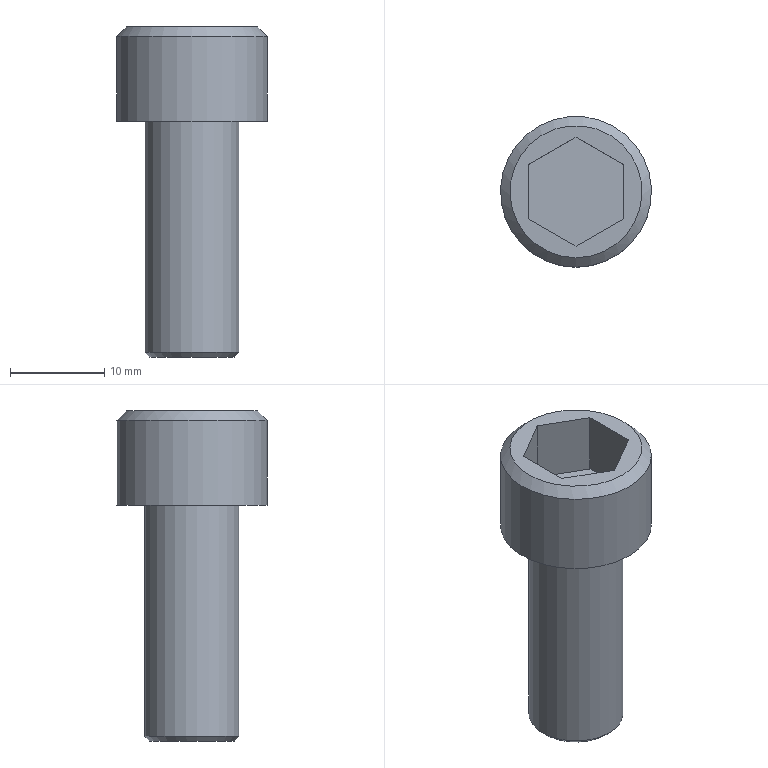Part | NX | features solid 2 | 1 solid | 14 faces | box 16 x 16 x 35 mm | volume 3369 mm3 | plane 10 | cylinder 2 | cone 2 | commonest cylinder face diameters 10 x1 16 x1
STEP:
#1=CARTESIAN_POINT('',(-54.,587.,-90.));
#2=VERTEX_POINT('',#1);
#3=CARTESIAN_POINT('',(-54.,595.,-90.));
#4=DIRECTION('',(0.,0.,1.));
#5=DIRECTION('',(0.,-1.,0.));
#6=AXIS2_PLACEMENT_3D('',#3,#4,#5);
#7=CIRCLE('',#6,8.);
#8=EDGE_CURVE('',#2,#2,#7,.F.);
#9=ORIENTED_EDGE('',*,*,#8,.T.);
#10=EDGE_LOOP('',(#9));
#11=FACE_BOUND('',#10,.T.);
#12=CARTESIAN_POINT('',(-54.,587.,-99.));
#13=VERTEX_POINT('',#12);
#14=CARTESIAN_POINT('',(-54.,595.,-99.));
#15=DIRECTION('',(0.,0.,1.));
#16=DIRECTION('',(0.,-1.,0.));
#17=AXIS2_PLACEMENT_3D('',#14,#15,#16);
#18=CIRCLE('',#17,8.);
#19=EDGE_CURVE('',#13,#13,#18,.T.);
#20=ORIENTED_EDGE('',*,*,#19,.T.);
#21=EDGE_LOOP('',(#20));
#22=FACE_BOUND('',#21,.T.);
#23=CARTESIAN_POINT('',(-54.,595.,-99.));
#24=DIRECTION('',(0.,0.,1.));
#25=DIRECTION('',(0.,-1.,0.));
#26=AXIS2_PLACEMENT_3D('',#23,#24,#25);
#27=CYLINDRICAL_SURFACE('',#26,8.);
#28=ADVANCED_FACE('',(#11,#22),#27,.T.);
#29=CARTESIAN_POINT('',(-54.,590.,-99.));
#30=VERTEX_POINT('',#29);
#31=CARTESIAN_POINT('',(-54.,595.,-99.));
#32=DIRECTION('',(0.,0.,1.));
#33=DIRECTION('',(0.,-1.,0.));
#34=AXIS2_PLACEMENT_3D('',#31,#32,#33);
#35=CIRCLE('',#34,5.);
#36=EDGE_CURVE('',#30,#30,#35,.F.);
#37=ORIENTED_EDGE('',*,*,#36,.F.);
#38=EDGE_LOOP('',(#37));
#39=FACE_BOUND('',#38,.T.);
#40=ORIENTED_EDGE('',*,*,#19,.F.);
#41=EDGE_LOOP('',(#40));
#42=FACE_BOUND('',#41,.T.);
#43=CARTESIAN_POINT('',(-54.,595.,-99.));
#44=DIRECTION('',(0.,0.,1.));
#45=DIRECTION('',(0.,-1.,0.));
#46=AXIS2_PLACEMENT_3D('',#43,#44,#45);
#47=PLANE('',#46);
#48=ADVANCED_FACE('',(#39,#42),#47,.F.);
#49=CARTESIAN_POINT('',(-54.,588.,-89.));
#50=VERTEX_POINT('',#49);
#51=CARTESIAN_POINT('',(-54.,595.,-89.));
#52=DIRECTION('',(0.,0.,1.));
#53=DIRECTION('',(0.,-1.,0.));
#54=AXIS2_PLACEMENT_3D('',#51,#52,#53);
#55=CIRCLE('',#54,7.);
#56=EDGE_CURVE('',#50,#50,#55,.T.);
#57=ORIENTED_EDGE('',*,*,#56,.T.);
#58=EDGE_LOOP('',(#57));
#59=FACE_BOUND('',#58,.T.);
#60=CARTESIAN_POINT('',(-49.,597.887,-89.));
#61=VERTEX_POINT('',#60);
#62=CARTESIAN_POINT('',(-54.,600.774,-89.));
#63=VERTEX_POINT('',#62);
#64=CARTESIAN_POINT('',(-49.,597.887,-89.));
#65=DIRECTION('',(-0.866,0.5,0.));
#66=VECTOR('',#65,1000.);
#67=LINE('',#64,#66);
#68=EDGE_CURVE('',#61,#63,#67,.T.);
#69=ORIENTED_EDGE('',*,*,#68,.F.);
#70=CARTESIAN_POINT('',(-49.,592.113,-89.));
#71=VERTEX_POINT('',#70);
#72=CARTESIAN_POINT('',(-49.,592.113,-89.));
#73=DIRECTION('',(0.,1.,0.));
#74=VECTOR('',#73,1000.);
#75=LINE('',#72,#74);
#76=EDGE_CURVE('',#71,#61,#75,.T.);
#77=ORIENTED_EDGE('',*,*,#76,.F.);
#78=CARTESIAN_POINT('',(-54.,589.226,-89.));
#79=VERTEX_POINT('',#78);
#80=CARTESIAN_POINT('',(-54.,589.226,-89.));
#81=DIRECTION('',(0.866,0.5,0.));
#82=VECTOR('',#81,1000.);
#83=LINE('',#80,#82);
#84=EDGE_CURVE('',#79,#71,#83,.T.);
#85=ORIENTED_EDGE('',*,*,#84,.F.);
#86=CARTESIAN_POINT('',(-59.,592.113,-89.));
#87=VERTEX_POINT('',#86);
#88=CARTESIAN_POINT('',(-59.,592.113,-89.));
#89=DIRECTION('',(0.866,-0.5,0.));
#90=VECTOR('',#89,1000.);
#91=LINE('',#88,#90);
#92=EDGE_CURVE('',#87,#79,#91,.T.);
#93=ORIENTED_EDGE('',*,*,#92,.F.);
#94=CARTESIAN_POINT('',(-59.,597.887,-89.));
#95=VERTEX_POINT('',#94);
#96=CARTESIAN_POINT('',(-59.,597.887,-89.));
#97=DIRECTION('',(0.,-1.,0.));
#98=VECTOR('',#97,1000.);
#99=LINE('',#96,#98);
#100=EDGE_CURVE('',#95,#87,#99,.T.);
#101=ORIENTED_EDGE('',*,*,#100,.F.);
#102=CARTESIAN_POINT('',(-54.,600.774,-89.));
#103=DIRECTION('',(-0.866,-0.5,0.));
#104=VECTOR('',#103,1000.);
#105=LINE('',#102,#104);
#106=EDGE_CURVE('',#63,#95,#105,.T.);
#107=ORIENTED_EDGE('',*,*,#106,.F.);
#108=EDGE_LOOP('',(#69,#77,#85,#93,#101,#107));
#109=FACE_BOUND('',#108,.T.);
#110=CARTESIAN_POINT('',(-54.,595.,-89.));
#111=DIRECTION('',(0.,0.,1.));
#112=DIRECTION('',(0.,-1.,0.));
#113=AXIS2_PLACEMENT_3D('',#110,#111,#112);
#114=PLANE('',#113);
#115=ADVANCED_FACE('',(#59,#109),#114,.T.);
#116=CARTESIAN_POINT('',(-54.,599.5,-124.));
#117=VERTEX_POINT('',#116);
#118=CARTESIAN_POINT('',(-54.,595.,-124.));
#119=DIRECTION('',(0.,0.,-1.));
#120=DIRECTION('',(0.,1.,0.));
#121=AXIS2_PLACEMENT_3D('',#118,#119,#120);
#122=CIRCLE('',#121,4.5);
#123=EDGE_CURVE('',#117,#117,#122,.T.);
#124=ORIENTED_EDGE('',*,*,#123,.T.);
#125=EDGE_LOOP('',(#124));
#126=FACE_BOUND('',#125,.T.);
#127=CARTESIAN_POINT('',(-54.,595.,-124.));
#128=DIRECTION('',(0.,0.,-1.));
#129=DIRECTION('',(0.,1.,0.));
#130=AXIS2_PLACEMENT_3D('',#127,#128,#129);
#131=PLANE('',#130);
#132=ADVANCED_FACE('',(#126),#131,.T.);
#133=CARTESIAN_POINT('',(-54.,600.,-123.5));
#134=VERTEX_POINT('',#133);
#135=CARTESIAN_POINT('',(-54.,595.,-123.5));
#136=DIRECTION('',(0.,0.,-1.));
#137=DIRECTION('',(0.,1.,0.));
#138=AXIS2_PLACEMENT_3D('',#135,#136,#137);
#139=CIRCLE('',#138,5.);
#140=EDGE_CURVE('',#134,#134,#139,.F.);
#141=ORIENTED_EDGE('',*,*,#140,.T.);
#142=EDGE_LOOP('',(#141));
#143=FACE_BOUND('',#142,.T.);
#144=ORIENTED_EDGE('',*,*,#36,.T.);
#145=EDGE_LOOP('',(#144));
#146=FACE_BOUND('',#145,.T.);
#147=CARTESIAN_POINT('',(-54.,595.,-89.));
#148=DIRECTION('',(0.,0.,-1.));
#149=DIRECTION('',(0.,1.,0.));
#150=AXIS2_PLACEMENT_3D('',#147,#148,#149);
#151=CYLINDRICAL_SURFACE('',#150,5.);
#152=ADVANCED_FACE('',(#143,#146),#151,.T.);
#153=ORIENTED_EDGE('',*,*,#68,.T.);
#154=CARTESIAN_POINT('',(-54.,600.774,-95.667));
#155=VERTEX_POINT('',#154);
#156=CARTESIAN_POINT('',(-54.,600.774,-95.667));
#157=DIRECTION('',(0.,0.,1.));
#158=VECTOR('',#157,1000.);
#159=LINE('',#156,#158);
#160=EDGE_CURVE('',#155,#63,#159,.T.);
#161=ORIENTED_EDGE('',*,*,#160,.F.);
#162=CARTESIAN_POINT('',(-49.,597.887,-95.667));
#163=VERTEX_POINT('',#162);
#164=CARTESIAN_POINT('',(-49.,597.887,-95.667));
#165=DIRECTION('',(-0.866,0.5,0.));
#166=VECTOR('',#165,1000.);
#167=LINE('',#164,#166);
#168=EDGE_CURVE('',#163,#155,#167,.T.);
#169=ORIENTED_EDGE('',*,*,#168,.F.);
#170=CARTESIAN_POINT('',(-49.,597.887,-95.667));
#171=DIRECTION('',(0.,0.,1.));
#172=VECTOR('',#171,1000.);
#173=LINE('',#170,#172);
#174=EDGE_CURVE('',#163,#61,#173,.T.);
#175=ORIENTED_EDGE('',*,*,#174,.T.);
#176=EDGE_LOOP('',(#153,#161,#169,#175));
#177=FACE_BOUND('',#176,.T.);
#178=CARTESIAN_POINT('',(-49.,597.887,-95.667));
#179=DIRECTION('',(0.5,0.866,0.));
#180=DIRECTION('',(-0.866,0.5,0.));
#181=AXIS2_PLACEMENT_3D('',#178,#179,#180);
#182=PLANE('',#181);
#183=ADVANCED_FACE('',(#177),#182,.F.);
#184=ORIENTED_EDGE('',*,*,#106,.T.);
#185=CARTESIAN_POINT('',(-59.,597.887,-95.667));
#186=VERTEX_POINT('',#185);
#187=CARTESIAN_POINT('',(-59.,597.887,-95.667));
#188=DIRECTION('',(0.,0.,1.));
#189=VECTOR('',#188,1000.);
#190=LINE('',#187,#189);
#191=EDGE_CURVE('',#186,#95,#190,.T.);
#192=ORIENTED_EDGE('',*,*,#191,.F.);
#193=CARTESIAN_POINT('',(-54.,600.774,-95.667));
#194=DIRECTION('',(-0.866,-0.5,0.));
#195=VECTOR('',#194,1000.);
#196=LINE('',#193,#195);
#197=EDGE_CURVE('',#155,#186,#196,.T.);
#198=ORIENTED_EDGE('',*,*,#197,.F.);
#199=ORIENTED_EDGE('',*,*,#160,.T.);
#200=EDGE_LOOP('',(#184,#192,#198,#199));
#201=FACE_BOUND('',#200,.T.);
#202=CARTESIAN_POINT('',(-54.,600.774,-95.667));
#203=DIRECTION('',(-0.5,0.866,0.));
#204=DIRECTION('',(-0.866,-0.5,0.));
#205=AXIS2_PLACEMENT_3D('',#202,#203,#204);
#206=PLANE('',#205);
#207=ADVANCED_FACE('',(#201),#206,.F.);
#208=ORIENTED_EDGE('',*,*,#100,.T.);
#209=CARTESIAN_POINT('',(-59.,592.113,-95.667));
#210=VERTEX_POINT('',#209);
#211=CARTESIAN_POINT('',(-59.,592.113,-95.667));
#212=DIRECTION('',(0.,0.,1.));
#213=VECTOR('',#212,1000.);
#214=LINE('',#211,#213);
#215=EDGE_CURVE('',#210,#87,#214,.T.);
#216=ORIENTED_EDGE('',*,*,#215,.F.);
#217=CARTESIAN_POINT('',(-59.,597.887,-95.667));
#218=DIRECTION('',(0.,-1.,0.));
#219=VECTOR('',#218,1000.);
#220=LINE('',#217,#219);
#221=EDGE_CURVE('',#186,#210,#220,.T.);
#222=ORIENTED_EDGE('',*,*,#221,.F.);
#223=ORIENTED_EDGE('',*,*,#191,.T.);
#224=EDGE_LOOP('',(#208,#216,#222,#223));
#225=FACE_BOUND('',#224,.T.);
#226=CARTESIAN_POINT('',(-59.,597.887,-95.667));
#227=DIRECTION('',(-1.,0.,0.));
#228=DIRECTION('',(0.,0.,-1.));
#229=AXIS2_PLACEMENT_3D('',#226,#227,#228);
#230=PLANE('',#229);
#231=ADVANCED_FACE('',(#225),#230,.F.);
#232=ORIENTED_EDGE('',*,*,#92,.T.);
#233=CARTESIAN_POINT('',(-54.,589.226,-95.667));
#234=VERTEX_POINT('',#233);
#235=CARTESIAN_POINT('',(-54.,589.226,-95.667));
#236=DIRECTION('',(0.,0.,1.));
#237=VECTOR('',#236,1000.);
#238=LINE('',#235,#237);
#239=EDGE_CURVE('',#234,#79,#238,.T.);
#240=ORIENTED_EDGE('',*,*,#239,.F.);
#241=CARTESIAN_POINT('',(-59.,592.113,-95.667));
#242=DIRECTION('',(0.866,-0.5,0.));
#243=VECTOR('',#242,1000.);
#244=LINE('',#241,#243);
#245=EDGE_CURVE('',#210,#234,#244,.T.);
#246=ORIENTED_EDGE('',*,*,#245,.F.);
#247=ORIENTED_EDGE('',*,*,#215,.T.);
#248=EDGE_LOOP('',(#232,#240,#246,#247));
#249=FACE_BOUND('',#248,.T.);
#250=CARTESIAN_POINT('',(-59.,592.113,-95.667));
#251=DIRECTION('',(-0.5,-0.866,0.));
#252=DIRECTION('',(0.866,-0.5,0.));
#253=AXIS2_PLACEMENT_3D('',#250,#251,#252);
#254=PLANE('',#253);
#255=ADVANCED_FACE('',(#249),#254,.F.);
#256=ORIENTED_EDGE('',*,*,#84,.T.);
#257=CARTESIAN_POINT('',(-49.,592.113,-95.667));
#258=VERTEX_POINT('',#257);
#259=CARTESIAN_POINT('',(-49.,592.113,-95.667));
#260=DIRECTION('',(0.,0.,1.));
#261=VECTOR('',#260,1000.);
#262=LINE('',#259,#261);
#263=EDGE_CURVE('',#258,#71,#262,.T.);
#264=ORIENTED_EDGE('',*,*,#263,.F.);
#265=CARTESIAN_POINT('',(-54.,589.226,-95.667));
#266=DIRECTION('',(0.866,0.5,0.));
#267=VECTOR('',#266,1000.);
#268=LINE('',#265,#267);
#269=EDGE_CURVE('',#234,#258,#268,.T.);
#270=ORIENTED_EDGE('',*,*,#269,.F.);
#271=ORIENTED_EDGE('',*,*,#239,.T.);
#272=EDGE_LOOP('',(#256,#264,#270,#271));
#273=FACE_BOUND('',#272,.T.);
#274=CARTESIAN_POINT('',(-54.,589.226,-95.667));
#275=DIRECTION('',(0.5,-0.866,0.));
#276=DIRECTION('',(0.866,0.5,0.));
#277=AXIS2_PLACEMENT_3D('',#274,#275,#276);
#278=PLANE('',#277);
#279=ADVANCED_FACE('',(#273),#278,.F.);
#280=ORIENTED_EDGE('',*,*,#76,.T.);
#281=ORIENTED_EDGE('',*,*,#174,.F.);
#282=CARTESIAN_POINT('',(-49.,592.113,-95.667));
#283=DIRECTION('',(0.,1.,0.));
#284=VECTOR('',#283,1000.);
#285=LINE('',#282,#284);
#286=EDGE_CURVE('',#258,#163,#285,.T.);
#287=ORIENTED_EDGE('',*,*,#286,.F.);
#288=ORIENTED_EDGE('',*,*,#263,.T.);
#289=EDGE_LOOP('',(#280,#281,#287,#288));
#290=FACE_BOUND('',#289,.T.);
#291=CARTESIAN_POINT('',(-49.,592.113,-95.667));
#292=DIRECTION('',(1.,0.,0.));
#293=DIRECTION('',(0.,1.,0.));
#294=AXIS2_PLACEMENT_3D('',#291,#292,#293);
#295=PLANE('',#294);
#296=ADVANCED_FACE('',(#290),#295,.F.);
#297=ORIENTED_EDGE('',*,*,#168,.T.);
#298=ORIENTED_EDGE('',*,*,#197,.T.);
#299=ORIENTED_EDGE('',*,*,#221,.T.);
#300=ORIENTED_EDGE('',*,*,#245,.T.);
#301=ORIENTED_EDGE('',*,*,#269,.T.);
#302=ORIENTED_EDGE('',*,*,#286,.T.);
#303=EDGE_LOOP('',(#297,#298,#299,#300,#301,#302));
#304=FACE_BOUND('',#303,.T.);
#305=CARTESIAN_POINT('',(-54.,600.774,-95.667));
#306=DIRECTION('',(0.,0.,1.));
#307=DIRECTION('',(0.,-1.,0.));
#308=AXIS2_PLACEMENT_3D('',#305,#306,#307);
#309=PLANE('',#308);
#310=ADVANCED_FACE('',(#304),#309,.T.);
#311=ORIENTED_EDGE('',*,*,#8,.F.);
#312=EDGE_LOOP('',(#311));
#313=FACE_BOUND('',#312,.T.);
#314=ORIENTED_EDGE('',*,*,#56,.F.);
#315=EDGE_LOOP('',(#314));
#316=FACE_BOUND('',#315,.T.);
#317=CARTESIAN_POINT('',(-54.,595.,-89.));
#318=DIRECTION('',(0.,0.,-1.));
#319=DIRECTION('',(0.,1.,0.));
#320=AXIS2_PLACEMENT_3D('',#317,#318,#319);
#321=CONICAL_SURFACE('',#320,7.,0.7854);
#322=ADVANCED_FACE('',(#313,#316),#321,.T.);
#323=ORIENTED_EDGE('',*,*,#140,.F.);
#324=EDGE_LOOP('',(#323));
#325=FACE_BOUND('',#324,.T.);
#326=ORIENTED_EDGE('',*,*,#123,.F.);
#327=EDGE_LOOP('',(#326));
#328=FACE_BOUND('',#327,.T.);
#329=CARTESIAN_POINT('',(-54.,595.,-124.));
#330=DIRECTION('',(0.,0.,1.));
#331=DIRECTION('',(0.,-1.,0.));
#332=AXIS2_PLACEMENT_3D('',#329,#330,#331);
#333=CONICAL_SURFACE('',#332,4.5,0.7854);
#334=ADVANCED_FACE('',(#325,#328),#333,.T.);
#335=CLOSED_SHELL('',(#28,#48,#115,#132,#152,#183,#207,#231,#255,#279,#296,#310,#322,#334));
#336=MANIFOLD_SOLID_BREP('',#335);
#337=(LENGTH_UNIT()NAMED_UNIT(*)SI_UNIT(.MILLI.,.METRE.));
#338=UNCERTAINTY_MEASURE_WITH_UNIT(LENGTH_MEASURE(0.00001),#337,'','');
#339=(NAMED_UNIT(*)PLANE_ANGLE_UNIT()SI_UNIT($,.RADIAN.));
#340=(NAMED_UNIT(*)SI_UNIT($,.STERADIAN.)SOLID_ANGLE_UNIT());
#341=(GEOMETRIC_REPRESENTATION_CONTEXT(3)GLOBAL_UNCERTAINTY_ASSIGNED_CONTEXT((#338))GLOBAL_UNIT_ASSIGNED_CONTEXT((#337,#339,#340))REPRESENTATION_CONTEXT('',''));
#342=ADVANCED_BREP_SHAPE_REPRESENTATION('',(#336),#341);